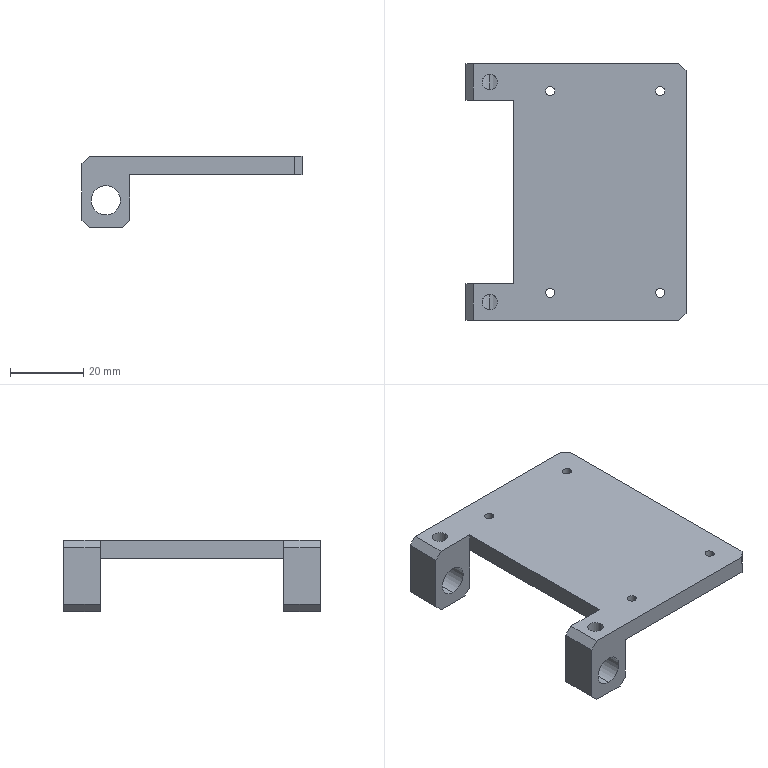Part | SolidWorks | features ICE 6, 3DProfileFeature 3, Chamfer 3, HoleWzd 3, Extrusion 1, LPattern 1 | 1 solid | 46 faces | box 60 x 70 x 19.5 mm | volume 20039 mm3 | plane 22 | cylinder 16 | cone 8 | commonest cylinder face diameters 2.5 x8 4.2 x4 8 x4